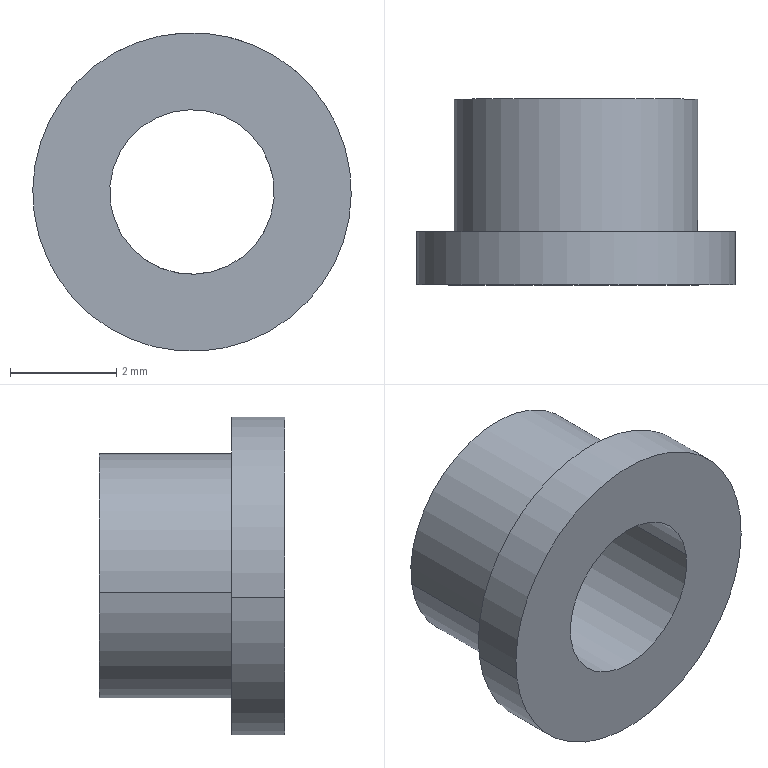Part | SolidWorks | features BaseBody 1 | 1 solid | 9 faces | box 6 x 3.502 x 6 mm | volume 43.405 mm3 | cylinder 6 | plane 3 | commonest cylinder face diameters 3.1 x2 4.6 x2 6 x2
STEP:
#1=CARTESIAN_POINT('',(-250.021,16.541,-40.895));
#2=VERTEX_POINT('',#1);
#3=CARTESIAN_POINT('',(-254.58,16.541,-41.509));
#4=VERTEX_POINT('',#3);
#5=CARTESIAN_POINT('',(-252.301,16.541,-41.202));
#6=DIRECTION('',(0.00003827,-1.,-0.0004455));
#7=DIRECTION('',(0.9911,-0.00002151,0.1334));
#8=AXIS2_PLACEMENT_3D('',#5,#6,#7);
#9=CIRCLE('',#8,2.3);
#10=EDGE_CURVE('',#2,#4,#9,.T.);
#11=ORIENTED_EDGE('',*,*,#10,.T.);
#12=CARTESIAN_POINT('',(-254.58,14.041,-41.51));
#13=VERTEX_POINT('',#12);
#14=CARTESIAN_POINT('',(-254.58,14.041,-41.51));
#15=DIRECTION('',(-0.00003827,1.,0.0004455));
#16=VECTOR('',#15,1000.);
#17=LINE('',#14,#16);
#18=EDGE_CURVE('',#13,#4,#17,.T.);
#19=ORIENTED_EDGE('',*,*,#18,.F.);
#20=CARTESIAN_POINT('',(-250.021,14.041,-40.896));
#21=VERTEX_POINT('',#20);
#22=CARTESIAN_POINT('',(-252.301,14.041,-41.203));
#23=DIRECTION('',(-0.00003827,1.,0.0004455));
#24=DIRECTION('',(-0.9911,0.00002151,-0.1334));
#25=AXIS2_PLACEMENT_3D('',#22,#23,#24);
#26=CIRCLE('',#25,2.3);
#27=EDGE_CURVE('',#13,#21,#26,.T.);
#28=ORIENTED_EDGE('',*,*,#27,.T.);
#29=CARTESIAN_POINT('',(-250.021,14.041,-40.896));
#30=DIRECTION('',(-0.00003827,1.,0.0004455));
#31=VECTOR('',#30,1000.);
#32=LINE('',#29,#31);
#33=EDGE_CURVE('',#21,#2,#32,.T.);
#34=ORIENTED_EDGE('',*,*,#33,.T.);
#35=EDGE_LOOP('',(#11,#19,#28,#34));
#36=FACE_OUTER_BOUND('',#35,.T.);
#37=CARTESIAN_POINT('',(-252.301,16.541,-41.202));
#38=DIRECTION('',(0.00003827,-1.,-0.0004455));
#39=DIRECTION('',(-0.9911,0.00002151,-0.1334));
#40=AXIS2_PLACEMENT_3D('',#37,#38,#39);
#41=CYLINDRICAL_SURFACE('',#40,2.3);
#42=ADVANCED_FACE('',(#36),#41,.T.);
#43=ORIENTED_EDGE('',*,*,#33,.F.);
#44=CARTESIAN_POINT('',(-252.301,14.041,-41.203));
#45=DIRECTION('',(-0.00003827,1.,0.0004455));
#46=DIRECTION('',(0.9911,-0.00002151,0.1334));
#47=AXIS2_PLACEMENT_3D('',#44,#45,#46);
#48=CIRCLE('',#47,2.3);
#49=EDGE_CURVE('',#21,#13,#48,.T.);
#50=ORIENTED_EDGE('',*,*,#49,.T.);
#51=ORIENTED_EDGE('',*,*,#18,.T.);
#52=CARTESIAN_POINT('',(-252.301,16.541,-41.202));
#53=DIRECTION('',(0.00003827,-1.,-0.0004455));
#54=DIRECTION('',(-0.9911,0.00002151,-0.1334));
#55=AXIS2_PLACEMENT_3D('',#52,#53,#54);
#56=CIRCLE('',#55,2.3);
#57=EDGE_CURVE('',#4,#2,#56,.T.);
#58=ORIENTED_EDGE('',*,*,#57,.T.);
#59=EDGE_LOOP('',(#43,#50,#51,#58));
#60=FACE_OUTER_BOUND('',#59,.T.);
#61=CARTESIAN_POINT('',(-252.301,16.541,-41.202));
#62=DIRECTION('',(0.00003827,-1.,-0.0004455));
#63=DIRECTION('',(-0.9911,0.00002151,-0.1334));
#64=AXIS2_PLACEMENT_3D('',#61,#62,#63);
#65=CYLINDRICAL_SURFACE('',#64,2.3);
#66=ADVANCED_FACE('',(#60),#65,.T.);
#67=CARTESIAN_POINT('',(-253.837,16.541,-41.409));
#68=VERTEX_POINT('',#67);
#69=CARTESIAN_POINT('',(-250.765,16.541,-40.995));
#70=VERTEX_POINT('',#69);
#71=CARTESIAN_POINT('',(-252.301,16.541,-41.202));
#72=DIRECTION('',(-0.00003827,1.,0.0004455));
#73=DIRECTION('',(-0.9911,0.00002151,-0.1334));
#74=AXIS2_PLACEMENT_3D('',#71,#72,#73);
#75=CIRCLE('',#74,1.55);
#76=EDGE_CURVE('',#68,#70,#75,.T.);
#77=ORIENTED_EDGE('',*,*,#76,.F.);
#78=CARTESIAN_POINT('',(-252.301,16.541,-41.202));
#79=DIRECTION('',(-0.00003827,1.,0.0004455));
#80=DIRECTION('',(0.9911,-0.00002151,0.1334));
#81=AXIS2_PLACEMENT_3D('',#78,#79,#80);
#82=CIRCLE('',#81,1.55);
#83=EDGE_CURVE('',#70,#68,#82,.T.);
#84=ORIENTED_EDGE('',*,*,#83,.F.);
#85=EDGE_LOOP('',(#77,#84));
#86=FACE_BOUND('',#85,.T.);
#87=ORIENTED_EDGE('',*,*,#57,.F.);
#88=ORIENTED_EDGE('',*,*,#10,.F.);
#89=EDGE_LOOP('',(#87,#88));
#90=FACE_OUTER_BOUND('',#89,.T.);
#91=CARTESIAN_POINT('',(-252.301,16.541,-41.202));
#92=DIRECTION('',(-0.00003827,1.,0.0004455));
#93=DIRECTION('',(0.9963,0.,0.08559));
#94=AXIS2_PLACEMENT_3D('',#91,#92,#93);
#95=PLANE('',#94);
#96=ADVANCED_FACE('',(#86,#90),#95,.T.);
#97=CARTESIAN_POINT('',(-253.837,13.041,-41.41));
#98=VERTEX_POINT('',#97);
#99=CARTESIAN_POINT('',(-250.764,13.041,-40.997));
#100=VERTEX_POINT('',#99);
#101=CARTESIAN_POINT('',(-252.301,13.041,-41.203));
#102=DIRECTION('',(0.00003827,-1.,-0.0004455));
#103=DIRECTION('',(-0.9911,0.00002151,-0.1334));
#104=AXIS2_PLACEMENT_3D('',#101,#102,#103);
#105=CIRCLE('',#104,1.55);
#106=EDGE_CURVE('',#98,#100,#105,.T.);
#107=ORIENTED_EDGE('',*,*,#106,.T.);
#108=CARTESIAN_POINT('',(-250.765,16.541,-40.995));
#109=DIRECTION('',(0.00003827,-1.,-0.0004455));
#110=VECTOR('',#109,1000.);
#111=LINE('',#108,#110);
#112=EDGE_CURVE('',#70,#100,#111,.T.);
#113=ORIENTED_EDGE('',*,*,#112,.F.);
#114=ORIENTED_EDGE('',*,*,#83,.T.);
#115=CARTESIAN_POINT('',(-253.837,16.541,-41.409));
#116=DIRECTION('',(0.00003827,-1.,-0.0004455));
#117=VECTOR('',#116,1000.);
#118=LINE('',#115,#117);
#119=EDGE_CURVE('',#68,#98,#118,.T.);
#120=ORIENTED_EDGE('',*,*,#119,.T.);
#121=EDGE_LOOP('',(#107,#113,#114,#120));
#122=FACE_OUTER_BOUND('',#121,.T.);
#123=CARTESIAN_POINT('',(-252.301,13.041,-41.203));
#124=DIRECTION('',(-0.00003827,1.,0.0004455));
#125=DIRECTION('',(0.9911,-0.00002151,0.1334));
#126=AXIS2_PLACEMENT_3D('',#123,#124,#125);
#127=CYLINDRICAL_SURFACE('',#126,1.55);
#128=ADVANCED_FACE('',(#122),#127,.F.);
#129=ORIENTED_EDGE('',*,*,#119,.F.);
#130=ORIENTED_EDGE('',*,*,#76,.T.);
#131=ORIENTED_EDGE('',*,*,#112,.T.);
#132=CARTESIAN_POINT('',(-252.301,13.041,-41.203));
#133=DIRECTION('',(0.00003827,-1.,-0.0004455));
#134=DIRECTION('',(0.9911,-0.00002151,0.1334));
#135=AXIS2_PLACEMENT_3D('',#132,#133,#134);
#136=CIRCLE('',#135,1.55);
#137=EDGE_CURVE('',#100,#98,#136,.T.);
#138=ORIENTED_EDGE('',*,*,#137,.T.);
#139=EDGE_LOOP('',(#129,#130,#131,#138));
#140=FACE_OUTER_BOUND('',#139,.T.);
#141=CARTESIAN_POINT('',(-252.301,13.041,-41.203));
#142=DIRECTION('',(-0.00003827,1.,0.0004455));
#143=DIRECTION('',(0.9911,-0.00002151,0.1334));
#144=AXIS2_PLACEMENT_3D('',#141,#142,#143);
#145=CYLINDRICAL_SURFACE('',#144,1.55);
#146=ADVANCED_FACE('',(#140),#145,.F.);
#147=ORIENTED_EDGE('',*,*,#137,.F.);
#148=ORIENTED_EDGE('',*,*,#106,.F.);
#149=EDGE_LOOP('',(#147,#148));
#150=FACE_BOUND('',#149,.T.);
#151=CARTESIAN_POINT('',(-249.327,13.041,-40.803));
#152=VERTEX_POINT('',#151);
#153=CARTESIAN_POINT('',(-255.274,13.041,-41.604));
#154=VERTEX_POINT('',#153);
#155=CARTESIAN_POINT('',(-252.301,13.041,-41.203));
#156=DIRECTION('',(-0.00003827,1.,0.0004455));
#157=DIRECTION('',(0.9911,-0.00002151,0.1334));
#158=AXIS2_PLACEMENT_3D('',#155,#156,#157);
#159=CIRCLE('',#158,3.);
#160=EDGE_CURVE('',#152,#154,#159,.T.);
#161=ORIENTED_EDGE('',*,*,#160,.F.);
#162=CARTESIAN_POINT('',(-252.301,13.041,-41.203));
#163=DIRECTION('',(-0.00003827,1.,0.0004455));
#164=DIRECTION('',(-0.9911,0.00002151,-0.1334));
#165=AXIS2_PLACEMENT_3D('',#162,#163,#164);
#166=CIRCLE('',#165,3.);
#167=EDGE_CURVE('',#154,#152,#166,.T.);
#168=ORIENTED_EDGE('',*,*,#167,.F.);
#169=EDGE_LOOP('',(#161,#168));
#170=FACE_OUTER_BOUND('',#169,.T.);
#171=CARTESIAN_POINT('',(-252.301,13.041,-41.203));
#172=DIRECTION('',(-0.00003827,1.,0.0004455));
#173=DIRECTION('',(0.9963,0.,0.08559));
#174=AXIS2_PLACEMENT_3D('',#171,#172,#173);
#175=PLANE('',#174);
#176=ADVANCED_FACE('',(#150,#170),#175,.F.);
#177=CARTESIAN_POINT('',(-249.327,14.041,-40.803));
#178=VERTEX_POINT('',#177);
#179=CARTESIAN_POINT('',(-255.274,14.041,-41.603));
#180=VERTEX_POINT('',#179);
#181=CARTESIAN_POINT('',(-252.301,14.041,-41.203));
#182=DIRECTION('',(0.00003827,-1.,-0.0004455));
#183=DIRECTION('',(0.9911,-0.00002151,0.1334));
#184=AXIS2_PLACEMENT_3D('',#181,#182,#183);
#185=CIRCLE('',#184,3.);
#186=EDGE_CURVE('',#178,#180,#185,.T.);
#187=ORIENTED_EDGE('',*,*,#186,.T.);
#188=CARTESIAN_POINT('',(-255.274,13.041,-41.604));
#189=DIRECTION('',(-0.00003827,1.,0.0004455));
#190=VECTOR('',#189,1000.);
#191=LINE('',#188,#190);
#192=EDGE_CURVE('',#154,#180,#191,.T.);
#193=ORIENTED_EDGE('',*,*,#192,.F.);
#194=ORIENTED_EDGE('',*,*,#167,.T.);
#195=CARTESIAN_POINT('',(-249.327,13.041,-40.803));
#196=DIRECTION('',(-0.00003827,1.,0.0004455));
#197=VECTOR('',#196,1000.);
#198=LINE('',#195,#197);
#199=EDGE_CURVE('',#152,#178,#198,.T.);
#200=ORIENTED_EDGE('',*,*,#199,.T.);
#201=EDGE_LOOP('',(#187,#193,#194,#200));
#202=FACE_OUTER_BOUND('',#201,.T.);
#203=CARTESIAN_POINT('',(-252.301,14.041,-41.203));
#204=DIRECTION('',(0.00003827,-1.,-0.0004455));
#205=DIRECTION('',(-0.9911,0.00002151,-0.1334));
#206=AXIS2_PLACEMENT_3D('',#203,#204,#205);
#207=CYLINDRICAL_SURFACE('',#206,3.);
#208=ADVANCED_FACE('',(#202),#207,.T.);
#209=ORIENTED_EDGE('',*,*,#199,.F.);
#210=ORIENTED_EDGE('',*,*,#160,.T.);
#211=ORIENTED_EDGE('',*,*,#192,.T.);
#212=CARTESIAN_POINT('',(-252.301,14.041,-41.203));
#213=DIRECTION('',(0.00003827,-1.,-0.0004455));
#214=DIRECTION('',(-0.9911,0.00002151,-0.1334));
#215=AXIS2_PLACEMENT_3D('',#212,#213,#214);
#216=CIRCLE('',#215,3.);
#217=EDGE_CURVE('',#180,#178,#216,.T.);
#218=ORIENTED_EDGE('',*,*,#217,.T.);
#219=EDGE_LOOP('',(#209,#210,#211,#218));
#220=FACE_OUTER_BOUND('',#219,.T.);
#221=CARTESIAN_POINT('',(-252.301,14.041,-41.203));
#222=DIRECTION('',(0.00003827,-1.,-0.0004455));
#223=DIRECTION('',(-0.9911,0.00002151,-0.1334));
#224=AXIS2_PLACEMENT_3D('',#221,#222,#223);
#225=CYLINDRICAL_SURFACE('',#224,3.);
#226=ADVANCED_FACE('',(#220),#225,.T.);
#227=ORIENTED_EDGE('',*,*,#49,.F.);
#228=ORIENTED_EDGE('',*,*,#27,.F.);
#229=EDGE_LOOP('',(#227,#228));
#230=FACE_BOUND('',#229,.T.);
#231=ORIENTED_EDGE('',*,*,#217,.F.);
#232=ORIENTED_EDGE('',*,*,#186,.F.);
#233=EDGE_LOOP('',(#231,#232));
#234=FACE_OUTER_BOUND('',#233,.T.);
#235=CARTESIAN_POINT('',(-252.301,14.041,-41.203));
#236=DIRECTION('',(-0.00003827,1.,0.0004455));
#237=DIRECTION('',(0.9963,0.,0.08559));
#238=AXIS2_PLACEMENT_3D('',#235,#236,#237);
#239=PLANE('',#238);
#240=ADVANCED_FACE('',(#230,#234),#239,.T.);
#241=CLOSED_SHELL('',(#42,#66,#96,#128,#146,#176,#208,#226,#240));
#242=MANIFOLD_SOLID_BREP('',#241);
#243=CARTESIAN_POINT('',(0.,0.,0.));
#244=DIRECTION('',(0.,0.,1.));
#245=DIRECTION('',(1.,0.,0.));
#246=AXIS2_PLACEMENT_3D('',#243,#244,#245);
#247=(LENGTH_UNIT()NAMED_UNIT(*)SI_UNIT(.MILLI.,.METRE.));
#248=UNCERTAINTY_MEASURE_WITH_UNIT(LENGTH_MEASURE(0.00001),#247,'','');
#249=(NAMED_UNIT(*)PLANE_ANGLE_UNIT()SI_UNIT($,.RADIAN.));
#250=(NAMED_UNIT(*)SI_UNIT($,.STERADIAN.)SOLID_ANGLE_UNIT());
#251=(GEOMETRIC_REPRESENTATION_CONTEXT(3)GLOBAL_UNCERTAINTY_ASSIGNED_CONTEXT((#248))GLOBAL_UNIT_ASSIGNED_CONTEXT((#247,#249,#250))REPRESENTATION_CONTEXT('',''));
#252=ADVANCED_BREP_SHAPE_REPRESENTATION('',(#242,#246),#251);